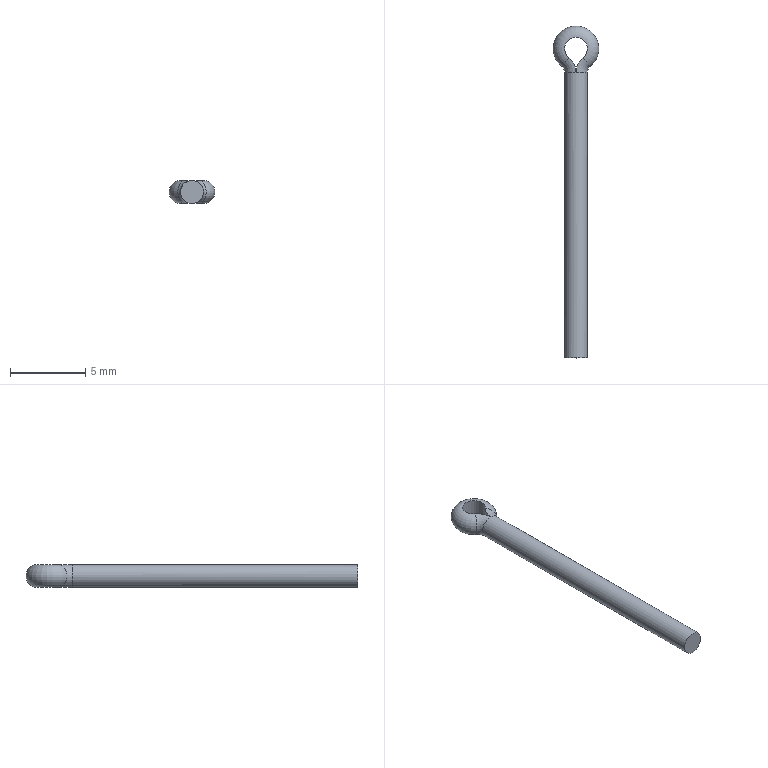Part | NX | features solid 2 | 1 solid | 8 faces | box 3.048 x 22.136 x 1.524 mm | volume 41.141 mm3 | cylinder 4 | torus 3 | plane 1 | commonest cylinder face diameters 1.524 x2 2.438 x2
STEP:
#1=CARTESIAN_POINT('',(-0.4689,20.011,-0.762));
#2=VERTEX_POINT('',#1);
#3=CARTESIAN_POINT('',(-0.4689,20.011,0.762));
#4=VERTEX_POINT('',#3);
#5=CARTESIAN_POINT('',(-0.4689,20.011,-0.762));
#6=DIRECTION('',(0.,0.,1.));
#7=VECTOR('',#6,1000.);
#8=LINE('',#5,#7);
#9=EDGE_CURVE('',#2,#4,#8,.T.);
#10=ORIENTED_EDGE('',*,*,#9,.F.);
#11=CARTESIAN_POINT('',(0.4689,20.011,-0.762));
#12=VERTEX_POINT('',#11);
#13=CARTESIAN_POINT('',(0.,20.612,-0.762));
#14=DIRECTION('',(0.,0.,-1.));
#15=DIRECTION('',(0.,1.,0.));
#16=AXIS2_PLACEMENT_3D('',#13,#14,#15);
#17=CIRCLE('',#16,0.762);
#18=EDGE_CURVE('',#2,#12,#17,.T.);
#19=ORIENTED_EDGE('',*,*,#18,.T.);
#20=CARTESIAN_POINT('',(0.4689,20.011,0.762));
#21=VERTEX_POINT('',#20);
#22=CARTESIAN_POINT('',(0.4689,20.011,-0.762));
#23=DIRECTION('',(0.,0.,1.));
#24=VECTOR('',#23,1000.);
#25=LINE('',#22,#24);
#26=EDGE_CURVE('',#12,#21,#25,.T.);
#27=ORIENTED_EDGE('',*,*,#26,.T.);
#28=CARTESIAN_POINT('',(0.,20.612,0.762));
#29=DIRECTION('',(0.,0.,-1.));
#30=DIRECTION('',(0.,1.,0.));
#31=AXIS2_PLACEMENT_3D('',#28,#29,#30);
#32=CIRCLE('',#31,0.762);
#33=EDGE_CURVE('',#21,#4,#32,.F.);
#34=ORIENTED_EDGE('',*,*,#33,.T.);
#35=EDGE_LOOP('',(#10,#19,#27,#34));
#36=FACE_BOUND('',#35,.T.);
#37=CARTESIAN_POINT('',(0.,20.612,0.));
#38=DIRECTION('',(0.,0.,-1.));
#39=DIRECTION('',(0.,1.,0.));
#40=AXIS2_PLACEMENT_3D('',#37,#38,#39);
#41=CYLINDRICAL_SURFACE('',#40,0.762);
#42=ADVANCED_FACE('',(#36),#41,.F.);
#43=CARTESIAN_POINT('',(-0.4689,20.011,0.));
#44=DIRECTION('',(0.7882,-0.6154,0.));
#45=DIRECTION('',(0.6154,0.7882,0.));
#46=AXIS2_PLACEMENT_3D('',#43,#44,#45);
#47=CIRCLE('',#46,0.762);
#48=EDGE_CURVE('',#4,#2,#47,.T.);
#49=ORIENTED_EDGE('',*,*,#48,.F.);
#50=ORIENTED_EDGE('',*,*,#33,.F.);
#51=CARTESIAN_POINT('',(0.4689,20.011,0.));
#52=DIRECTION('',(0.7882,0.6154,0.));
#53=DIRECTION('',(-0.6154,0.7882,0.));
#54=AXIS2_PLACEMENT_3D('',#51,#52,#53);
#55=CIRCLE('',#54,0.762);
#56=EDGE_CURVE('',#21,#12,#55,.T.);
#57=ORIENTED_EDGE('',*,*,#56,.T.);
#58=ORIENTED_EDGE('',*,*,#18,.F.);
#59=EDGE_LOOP('',(#49,#50,#57,#58));
#60=FACE_BOUND('',#59,.T.);
#61=CARTESIAN_POINT('',(0.,20.612,0.));
#62=DIRECTION('',(0.,0.,-1.));
#63=DIRECTION('',(0.,1.,0.));
#64=AXIS2_PLACEMENT_3D('',#61,#62,#63);
#65=TOROIDAL_SURFACE('',#64,0.762,0.762);
#66=ADVANCED_FACE('',(#60),#65,.T.);
#67=CARTESIAN_POINT('',(0.,19.05,-0.762));
#68=VERTEX_POINT('',#67);
#69=CARTESIAN_POINT('',(0.,19.05,0.762));
#70=VERTEX_POINT('',#69);
#71=CARTESIAN_POINT('',(0.,19.05,-0.762));
#72=DIRECTION('',(0.,0.,1.));
#73=VECTOR('',#72,1000.);
#74=LINE('',#71,#73);
#75=EDGE_CURVE('',#68,#70,#74,.T.);
#76=ORIENTED_EDGE('',*,*,#75,.F.);
#77=CARTESIAN_POINT('',(-1.219,19.05,-0.762));
#78=DIRECTION('',(0.,0.,1.));
#79=DIRECTION('',(0.,-1.,0.));
#80=AXIS2_PLACEMENT_3D('',#77,#78,#79);
#81=CIRCLE('',#80,1.219);
#82=EDGE_CURVE('',#2,#68,#81,.F.);
#83=ORIENTED_EDGE('',*,*,#82,.F.);
#84=ORIENTED_EDGE('',*,*,#9,.T.);
#85=CARTESIAN_POINT('',(-1.219,19.05,0.762));
#86=DIRECTION('',(0.,0.,1.));
#87=DIRECTION('',(0.,-1.,0.));
#88=AXIS2_PLACEMENT_3D('',#85,#86,#87);
#89=CIRCLE('',#88,1.219);
#90=EDGE_CURVE('',#70,#4,#89,.T.);
#91=ORIENTED_EDGE('',*,*,#90,.F.);
#92=EDGE_LOOP('',(#76,#83,#84,#91));
#93=FACE_BOUND('',#92,.T.);
#94=CARTESIAN_POINT('',(-1.219,19.05,0.));
#95=DIRECTION('',(0.,0.,1.));
#96=DIRECTION('',(0.,-1.,0.));
#97=AXIS2_PLACEMENT_3D('',#94,#95,#96);
#98=CYLINDRICAL_SURFACE('',#97,1.219);
#99=ADVANCED_FACE('',(#93),#98,.T.);
#100=CARTESIAN_POINT('',(0.,19.05,0.));
#101=DIRECTION('',(0.,-1.,0.));
#102=DIRECTION('',(1.,0.,0.));
#103=AXIS2_PLACEMENT_3D('',#100,#101,#102);
#104=CIRCLE('',#103,0.762);
#105=EDGE_CURVE('',#70,#68,#104,.T.);
#106=ORIENTED_EDGE('',*,*,#105,.F.);
#107=ORIENTED_EDGE('',*,*,#90,.T.);
#108=ORIENTED_EDGE('',*,*,#48,.T.);
#109=ORIENTED_EDGE('',*,*,#82,.T.);
#110=EDGE_LOOP('',(#106,#107,#108,#109));
#111=FACE_BOUND('',#110,.T.);
#112=CARTESIAN_POINT('',(-1.219,19.05,0.));
#113=DIRECTION('',(0.,0.,1.));
#114=DIRECTION('',(0.,-1.,0.));
#115=AXIS2_PLACEMENT_3D('',#112,#113,#114);
#116=TOROIDAL_SURFACE('',#115,1.219,0.762);
#117=ADVANCED_FACE('',(#111),#116,.T.);
#118=CARTESIAN_POINT('',(0.762,0.,0.));
#119=VERTEX_POINT('',#118);
#120=CARTESIAN_POINT('',(0.,0.,0.));
#121=DIRECTION('',(0.,-1.,0.));
#122=DIRECTION('',(1.,0.,0.));
#123=AXIS2_PLACEMENT_3D('',#120,#121,#122);
#124=CIRCLE('',#123,0.762);
#125=EDGE_CURVE('',#119,#119,#124,.T.);
#126=ORIENTED_EDGE('',*,*,#125,.F.);
#127=EDGE_LOOP('',(#126));
#128=FACE_BOUND('',#127,.T.);
#129=CARTESIAN_POINT('',(0.,19.05,0.));
#130=DIRECTION('',(0.,1.,0.));
#131=DIRECTION('',(-1.,0.,0.));
#132=AXIS2_PLACEMENT_3D('',#129,#130,#131);
#133=CIRCLE('',#132,0.762);
#134=EDGE_CURVE('',#68,#70,#133,.F.);
#135=ORIENTED_EDGE('',*,*,#134,.T.);
#136=ORIENTED_EDGE('',*,*,#105,.T.);
#137=EDGE_LOOP('',(#135,#136));
#138=FACE_BOUND('',#137,.T.);
#139=CARTESIAN_POINT('',(0.,19.05,0.));
#140=DIRECTION('',(0.,-1.,0.));
#141=DIRECTION('',(0.,0.,-1.));
#142=AXIS2_PLACEMENT_3D('',#139,#140,#141);
#143=CYLINDRICAL_SURFACE('',#142,0.762);
#144=ADVANCED_FACE('',(#128,#138),#143,.T.);
#145=ORIENTED_EDGE('',*,*,#125,.T.);
#146=EDGE_LOOP('',(#145));
#147=FACE_BOUND('',#146,.T.);
#148=CARTESIAN_POINT('',(0.,0.,0.));
#149=DIRECTION('',(0.,-1.,0.));
#150=DIRECTION('',(0.,0.,-1.));
#151=AXIS2_PLACEMENT_3D('',#148,#149,#150);
#152=PLANE('',#151);
#153=ADVANCED_FACE('',(#147),#152,.T.);
#154=ORIENTED_EDGE('',*,*,#75,.T.);
#155=CARTESIAN_POINT('',(1.219,19.05,0.762));
#156=DIRECTION('',(0.,0.,-1.));
#157=DIRECTION('',(0.,-1.,0.));
#158=AXIS2_PLACEMENT_3D('',#155,#156,#157);
#159=CIRCLE('',#158,1.219);
#160=EDGE_CURVE('',#70,#21,#159,.T.);
#161=ORIENTED_EDGE('',*,*,#160,.T.);
#162=ORIENTED_EDGE('',*,*,#26,.F.);
#163=CARTESIAN_POINT('',(1.219,19.05,-0.762));
#164=DIRECTION('',(0.,0.,-1.));
#165=DIRECTION('',(0.,-1.,0.));
#166=AXIS2_PLACEMENT_3D('',#163,#164,#165);
#167=CIRCLE('',#166,1.219);
#168=EDGE_CURVE('',#12,#68,#167,.F.);
#169=ORIENTED_EDGE('',*,*,#168,.T.);
#170=EDGE_LOOP('',(#154,#161,#162,#169));
#171=FACE_BOUND('',#170,.T.);
#172=CARTESIAN_POINT('',(1.219,19.05,0.));
#173=DIRECTION('',(0.,0.,1.));
#174=DIRECTION('',(0.,-1.,0.));
#175=AXIS2_PLACEMENT_3D('',#172,#173,#174);
#176=CYLINDRICAL_SURFACE('',#175,1.219);
#177=ADVANCED_FACE('',(#171),#176,.T.);
#178=ORIENTED_EDGE('',*,*,#134,.F.);
#179=ORIENTED_EDGE('',*,*,#168,.F.);
#180=ORIENTED_EDGE('',*,*,#56,.F.);
#181=ORIENTED_EDGE('',*,*,#160,.F.);
#182=EDGE_LOOP('',(#178,#179,#180,#181));
#183=FACE_BOUND('',#182,.T.);
#184=CARTESIAN_POINT('',(1.219,19.05,0.));
#185=DIRECTION('',(0.,0.,1.));
#186=DIRECTION('',(0.,-1.,0.));
#187=AXIS2_PLACEMENT_3D('',#184,#185,#186);
#188=TOROIDAL_SURFACE('',#187,1.219,0.762);
#189=ADVANCED_FACE('',(#183),#188,.T.);
#190=CLOSED_SHELL('',(#42,#66,#99,#117,#144,#153,#177,#189));
#191=MANIFOLD_SOLID_BREP('',#190);
#192=(LENGTH_UNIT()NAMED_UNIT(*)SI_UNIT(.MILLI.,.METRE.));
#193=UNCERTAINTY_MEASURE_WITH_UNIT(LENGTH_MEASURE(0.00001),#192,'','');
#194=(NAMED_UNIT(*)PLANE_ANGLE_UNIT()SI_UNIT($,.RADIAN.));
#195=(NAMED_UNIT(*)SI_UNIT($,.STERADIAN.)SOLID_ANGLE_UNIT());
#196=(GEOMETRIC_REPRESENTATION_CONTEXT(3)GLOBAL_UNCERTAINTY_ASSIGNED_CONTEXT((#193))GLOBAL_UNIT_ASSIGNED_CONTEXT((#192,#194,#195))REPRESENTATION_CONTEXT('',''));
#197=ADVANCED_BREP_SHAPE_REPRESENTATION('',(#191),#196);